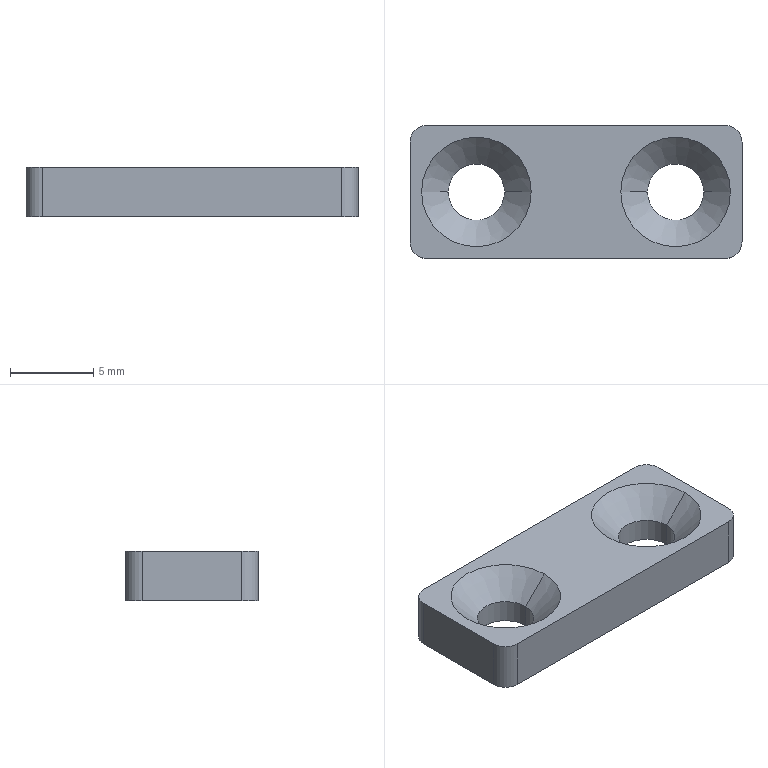Part | STEP file | 03-19 sensor press plate | 1 solid | 18 faces | box 20 x 8 x 3 mm | volume 387.026 mm3 | cylinder 8 | plane 6 | cone 4 | commonest cylinder face diameters 2 x4 3.4 x4
STEP:
#1=CARTESIAN_POINT('',(-7.7,0.,1.4));
#2=VERTEX_POINT('',#1);
#3=CARTESIAN_POINT('',(-4.3,0.,1.4));
#4=VERTEX_POINT('',#3);
#5=CARTESIAN_POINT('',(-6.,0.,1.4));
#6=DIRECTION('',(0.,0.,1.));
#7=DIRECTION('',(1.,0.,0.));
#8=AXIS2_PLACEMENT_3D('',#5,#6,#7);
#9=CIRCLE('',#8,1.7);
#10=EDGE_CURVE('',#2,#4,#9,.T.);
#11=ORIENTED_EDGE('',*,*,#10,.F.);
#12=CARTESIAN_POINT('',(-9.3,0.,3.));
#13=VERTEX_POINT('',#12);
#14=CARTESIAN_POINT('',(-9.3,0.,3.));
#15=DIRECTION('',(-0.7071,0.,0.7071));
#16=VECTOR('',#15,1000.);
#17=LINE('',#14,#16);
#18=EDGE_CURVE('',#2,#13,#17,.T.);
#19=ORIENTED_EDGE('',*,*,#18,.T.);
#20=CARTESIAN_POINT('',(-2.7,0.,3.));
#21=VERTEX_POINT('',#20);
#22=CARTESIAN_POINT('',(-6.,0.,3.));
#23=DIRECTION('',(0.,0.,1.));
#24=DIRECTION('',(1.,0.,0.));
#25=AXIS2_PLACEMENT_3D('',#22,#23,#24);
#26=CIRCLE('',#25,3.3);
#27=EDGE_CURVE('',#13,#21,#26,.T.);
#28=ORIENTED_EDGE('',*,*,#27,.T.);
#29=CARTESIAN_POINT('',(-2.7,0.,3.));
#30=DIRECTION('',(0.7071,0.,0.7071));
#31=VECTOR('',#30,1000.);
#32=LINE('',#29,#31);
#33=EDGE_CURVE('',#4,#21,#32,.T.);
#34=ORIENTED_EDGE('',*,*,#33,.F.);
#35=EDGE_LOOP('',(#11,#19,#28,#34));
#36=FACE_OUTER_BOUND('',#35,.T.);
#37=CARTESIAN_POINT('',(-6.,0.,3.));
#38=DIRECTION('',(0.,0.,1.));
#39=DIRECTION('',(1.,0.,0.));
#40=AXIS2_PLACEMENT_3D('',#37,#38,#39);
#41=CONICAL_SURFACE('',#40,3.3,0.7854);
#42=ADVANCED_FACE('',(#36),#41,.F.);
#43=CARTESIAN_POINT('',(-7.7,0.,0.));
#44=VERTEX_POINT('',#43);
#45=CARTESIAN_POINT('',(-4.3,0.,0.));
#46=VERTEX_POINT('',#45);
#47=CARTESIAN_POINT('',(-6.,0.,0.));
#48=DIRECTION('',(0.,0.,1.));
#49=DIRECTION('',(1.,0.,0.));
#50=AXIS2_PLACEMENT_3D('',#47,#48,#49);
#51=CIRCLE('',#50,1.7);
#52=EDGE_CURVE('',#44,#46,#51,.T.);
#53=ORIENTED_EDGE('',*,*,#52,.F.);
#54=CARTESIAN_POINT('',(-7.7,0.,3.));
#55=DIRECTION('',(0.,0.,1.));
#56=VECTOR('',#55,1000.);
#57=LINE('',#54,#56);
#58=EDGE_CURVE('',#44,#2,#57,.T.);
#59=ORIENTED_EDGE('',*,*,#58,.T.);
#60=ORIENTED_EDGE('',*,*,#10,.T.);
#61=CARTESIAN_POINT('',(-4.3,0.,3.));
#62=DIRECTION('',(0.,0.,1.));
#63=VECTOR('',#62,1000.);
#64=LINE('',#61,#63);
#65=EDGE_CURVE('',#46,#4,#64,.T.);
#66=ORIENTED_EDGE('',*,*,#65,.F.);
#67=EDGE_LOOP('',(#53,#59,#60,#66));
#68=FACE_OUTER_BOUND('',#67,.T.);
#69=CARTESIAN_POINT('',(-6.,0.,3.));
#70=DIRECTION('',(0.,0.,1.));
#71=DIRECTION('',(1.,0.,0.));
#72=AXIS2_PLACEMENT_3D('',#69,#70,#71);
#73=CYLINDRICAL_SURFACE('',#72,1.7);
#74=ADVANCED_FACE('',(#68),#73,.F.);
#75=CARTESIAN_POINT('',(4.3,0.,1.4));
#76=VERTEX_POINT('',#75);
#77=CARTESIAN_POINT('',(7.7,0.,1.4));
#78=VERTEX_POINT('',#77);
#79=CARTESIAN_POINT('',(6.,0.,1.4));
#80=DIRECTION('',(0.,0.,1.));
#81=DIRECTION('',(1.,0.,0.));
#82=AXIS2_PLACEMENT_3D('',#79,#80,#81);
#83=CIRCLE('',#82,1.7);
#84=EDGE_CURVE('',#76,#78,#83,.T.);
#85=ORIENTED_EDGE('',*,*,#84,.F.);
#86=CARTESIAN_POINT('',(2.7,0.,3.));
#87=VERTEX_POINT('',#86);
#88=CARTESIAN_POINT('',(2.7,0.,3.));
#89=DIRECTION('',(-0.7071,0.,0.7071));
#90=VECTOR('',#89,1000.);
#91=LINE('',#88,#90);
#92=EDGE_CURVE('',#76,#87,#91,.T.);
#93=ORIENTED_EDGE('',*,*,#92,.T.);
#94=CARTESIAN_POINT('',(9.3,0.,3.));
#95=VERTEX_POINT('',#94);
#96=CARTESIAN_POINT('',(6.,0.,3.));
#97=DIRECTION('',(0.,0.,1.));
#98=DIRECTION('',(1.,0.,0.));
#99=AXIS2_PLACEMENT_3D('',#96,#97,#98);
#100=CIRCLE('',#99,3.3);
#101=EDGE_CURVE('',#87,#95,#100,.T.);
#102=ORIENTED_EDGE('',*,*,#101,.T.);
#103=CARTESIAN_POINT('',(9.3,0.,3.));
#104=DIRECTION('',(0.7071,0.,0.7071));
#105=VECTOR('',#104,1000.);
#106=LINE('',#103,#105);
#107=EDGE_CURVE('',#78,#95,#106,.T.);
#108=ORIENTED_EDGE('',*,*,#107,.F.);
#109=EDGE_LOOP('',(#85,#93,#102,#108));
#110=FACE_OUTER_BOUND('',#109,.T.);
#111=CARTESIAN_POINT('',(6.,0.,3.));
#112=DIRECTION('',(0.,0.,1.));
#113=DIRECTION('',(1.,0.,0.));
#114=AXIS2_PLACEMENT_3D('',#111,#112,#113);
#115=CONICAL_SURFACE('',#114,3.3,0.7854);
#116=ADVANCED_FACE('',(#110),#115,.F.);
#117=CARTESIAN_POINT('',(4.3,0.,0.));
#118=VERTEX_POINT('',#117);
#119=CARTESIAN_POINT('',(7.7,0.,0.));
#120=VERTEX_POINT('',#119);
#121=CARTESIAN_POINT('',(6.,0.,0.));
#122=DIRECTION('',(0.,0.,1.));
#123=DIRECTION('',(1.,0.,0.));
#124=AXIS2_PLACEMENT_3D('',#121,#122,#123);
#125=CIRCLE('',#124,1.7);
#126=EDGE_CURVE('',#118,#120,#125,.T.);
#127=ORIENTED_EDGE('',*,*,#126,.F.);
#128=CARTESIAN_POINT('',(4.3,0.,3.));
#129=DIRECTION('',(0.,0.,1.));
#130=VECTOR('',#129,1000.);
#131=LINE('',#128,#130);
#132=EDGE_CURVE('',#118,#76,#131,.T.);
#133=ORIENTED_EDGE('',*,*,#132,.T.);
#134=ORIENTED_EDGE('',*,*,#84,.T.);
#135=CARTESIAN_POINT('',(7.7,0.,3.));
#136=DIRECTION('',(0.,0.,1.));
#137=VECTOR('',#136,1000.);
#138=LINE('',#135,#137);
#139=EDGE_CURVE('',#120,#78,#138,.T.);
#140=ORIENTED_EDGE('',*,*,#139,.F.);
#141=EDGE_LOOP('',(#127,#133,#134,#140));
#142=FACE_OUTER_BOUND('',#141,.T.);
#143=CARTESIAN_POINT('',(6.,0.,3.));
#144=DIRECTION('',(0.,0.,1.));
#145=DIRECTION('',(1.,0.,0.));
#146=AXIS2_PLACEMENT_3D('',#143,#144,#145);
#147=CYLINDRICAL_SURFACE('',#146,1.7);
#148=ADVANCED_FACE('',(#142),#147,.F.);
#149=CARTESIAN_POINT('',(10.,-3.,3.));
#150=VERTEX_POINT('',#149);
#151=CARTESIAN_POINT('',(10.,3.,3.));
#152=VERTEX_POINT('',#151);
#153=CARTESIAN_POINT('',(10.,4.,3.));
#154=DIRECTION('',(0.,1.,0.));
#155=VECTOR('',#154,1000.);
#156=LINE('',#153,#155);
#157=EDGE_CURVE('',#150,#152,#156,.T.);
#158=ORIENTED_EDGE('',*,*,#157,.F.);
#159=CARTESIAN_POINT('',(10.,-3.,0.));
#160=VERTEX_POINT('',#159);
#161=CARTESIAN_POINT('',(10.,-3.,3.));
#162=DIRECTION('',(0.,0.,-1.));
#163=VECTOR('',#162,1000.);
#164=LINE('',#161,#163);
#165=EDGE_CURVE('',#150,#160,#164,.T.);
#166=ORIENTED_EDGE('',*,*,#165,.T.);
#167=CARTESIAN_POINT('',(10.,3.,0.));
#168=VERTEX_POINT('',#167);
#169=CARTESIAN_POINT('',(10.,4.,0.));
#170=DIRECTION('',(0.,1.,0.));
#171=VECTOR('',#170,1000.);
#172=LINE('',#169,#171);
#173=EDGE_CURVE('',#160,#168,#172,.T.);
#174=ORIENTED_EDGE('',*,*,#173,.T.);
#175=CARTESIAN_POINT('',(10.,3.,3.));
#176=DIRECTION('',(0.,0.,1.));
#177=VECTOR('',#176,1000.);
#178=LINE('',#175,#177);
#179=EDGE_CURVE('',#168,#152,#178,.T.);
#180=ORIENTED_EDGE('',*,*,#179,.T.);
#181=EDGE_LOOP('',(#158,#166,#174,#180));
#182=FACE_OUTER_BOUND('',#181,.T.);
#183=CARTESIAN_POINT('',(10.,4.,3.));
#184=DIRECTION('',(-1.,0.,0.));
#185=DIRECTION('',(0.,-1.,0.));
#186=AXIS2_PLACEMENT_3D('',#183,#184,#185);
#187=PLANE('',#186);
#188=ADVANCED_FACE('',(#182),#187,.F.);
#189=CARTESIAN_POINT('',(9.,4.,3.));
#190=VERTEX_POINT('',#189);
#191=CARTESIAN_POINT('',(-9.,4.,3.));
#192=VERTEX_POINT('',#191);
#193=CARTESIAN_POINT('',(-10.,4.,3.));
#194=DIRECTION('',(-1.,0.,0.));
#195=VECTOR('',#194,1000.);
#196=LINE('',#193,#195);
#197=EDGE_CURVE('',#190,#192,#196,.T.);
#198=ORIENTED_EDGE('',*,*,#197,.F.);
#199=CARTESIAN_POINT('',(9.,4.,0.));
#200=VERTEX_POINT('',#199);
#201=CARTESIAN_POINT('',(9.,4.,3.));
#202=DIRECTION('',(0.,0.,-1.));
#203=VECTOR('',#202,1000.);
#204=LINE('',#201,#203);
#205=EDGE_CURVE('',#190,#200,#204,.T.);
#206=ORIENTED_EDGE('',*,*,#205,.T.);
#207=CARTESIAN_POINT('',(-9.,4.,0.));
#208=VERTEX_POINT('',#207);
#209=CARTESIAN_POINT('',(-10.,4.,0.));
#210=DIRECTION('',(-1.,0.,0.));
#211=VECTOR('',#210,1000.);
#212=LINE('',#209,#211);
#213=EDGE_CURVE('',#200,#208,#212,.T.);
#214=ORIENTED_EDGE('',*,*,#213,.T.);
#215=CARTESIAN_POINT('',(-9.,4.,3.));
#216=DIRECTION('',(0.,0.,1.));
#217=VECTOR('',#216,1000.);
#218=LINE('',#215,#217);
#219=EDGE_CURVE('',#208,#192,#218,.T.);
#220=ORIENTED_EDGE('',*,*,#219,.T.);
#221=EDGE_LOOP('',(#198,#206,#214,#220));
#222=FACE_OUTER_BOUND('',#221,.T.);
#223=CARTESIAN_POINT('',(-10.,4.,3.));
#224=DIRECTION('',(0.,-1.,0.));
#225=DIRECTION('',(0.,0.,-1.));
#226=AXIS2_PLACEMENT_3D('',#223,#224,#225);
#227=PLANE('',#226);
#228=ADVANCED_FACE('',(#222),#227,.F.);
#229=CARTESIAN_POINT('',(-10.,3.,0.));
#230=VERTEX_POINT('',#229);
#231=CARTESIAN_POINT('',(-10.,-3.,0.));
#232=VERTEX_POINT('',#231);
#233=CARTESIAN_POINT('',(-10.,4.,0.));
#234=DIRECTION('',(0.,-1.,0.));
#235=VECTOR('',#234,1000.);
#236=LINE('',#233,#235);
#237=EDGE_CURVE('',#230,#232,#236,.T.);
#238=ORIENTED_EDGE('',*,*,#237,.T.);
#239=CARTESIAN_POINT('',(-10.,-3.,3.));
#240=VERTEX_POINT('',#239);
#241=CARTESIAN_POINT('',(-10.,-3.,3.));
#242=DIRECTION('',(0.,0.,1.));
#243=VECTOR('',#242,1000.);
#244=LINE('',#241,#243);
#245=EDGE_CURVE('',#232,#240,#244,.T.);
#246=ORIENTED_EDGE('',*,*,#245,.T.);
#247=CARTESIAN_POINT('',(-10.,3.,3.));
#248=VERTEX_POINT('',#247);
#249=CARTESIAN_POINT('',(-10.,4.,3.));
#250=DIRECTION('',(0.,-1.,0.));
#251=VECTOR('',#250,1000.);
#252=LINE('',#249,#251);
#253=EDGE_CURVE('',#248,#240,#252,.T.);
#254=ORIENTED_EDGE('',*,*,#253,.F.);
#255=CARTESIAN_POINT('',(-10.,3.,3.));
#256=DIRECTION('',(0.,0.,-1.));
#257=VECTOR('',#256,1000.);
#258=LINE('',#255,#257);
#259=EDGE_CURVE('',#248,#230,#258,.T.);
#260=ORIENTED_EDGE('',*,*,#259,.T.);
#261=EDGE_LOOP('',(#238,#246,#254,#260));
#262=FACE_OUTER_BOUND('',#261,.T.);
#263=CARTESIAN_POINT('',(-10.,4.,3.));
#264=DIRECTION('',(1.,0.,0.));
#265=DIRECTION('',(0.,1.,0.));
#266=AXIS2_PLACEMENT_3D('',#263,#264,#265);
#267=PLANE('',#266);
#268=ADVANCED_FACE('',(#262),#267,.F.);
#269=CARTESIAN_POINT('',(-9.,-4.,0.));
#270=VERTEX_POINT('',#269);
#271=CARTESIAN_POINT('',(9.,-4.,0.));
#272=VERTEX_POINT('',#271);
#273=CARTESIAN_POINT('',(-10.,-4.,0.));
#274=DIRECTION('',(1.,0.,0.));
#275=VECTOR('',#274,1000.);
#276=LINE('',#273,#275);
#277=EDGE_CURVE('',#270,#272,#276,.T.);
#278=ORIENTED_EDGE('',*,*,#277,.T.);
#279=CARTESIAN_POINT('',(9.,-4.,3.));
#280=VERTEX_POINT('',#279);
#281=CARTESIAN_POINT('',(9.,-4.,3.));
#282=DIRECTION('',(0.,0.,1.));
#283=VECTOR('',#282,1000.);
#284=LINE('',#281,#283);
#285=EDGE_CURVE('',#272,#280,#284,.T.);
#286=ORIENTED_EDGE('',*,*,#285,.T.);
#287=CARTESIAN_POINT('',(-9.,-4.,3.));
#288=VERTEX_POINT('',#287);
#289=CARTESIAN_POINT('',(-10.,-4.,3.));
#290=DIRECTION('',(1.,0.,0.));
#291=VECTOR('',#290,1000.);
#292=LINE('',#289,#291);
#293=EDGE_CURVE('',#288,#280,#292,.T.);
#294=ORIENTED_EDGE('',*,*,#293,.F.);
#295=CARTESIAN_POINT('',(-9.,-4.,3.));
#296=DIRECTION('',(0.,0.,-1.));
#297=VECTOR('',#296,1000.);
#298=LINE('',#295,#297);
#299=EDGE_CURVE('',#288,#270,#298,.T.);
#300=ORIENTED_EDGE('',*,*,#299,.T.);
#301=EDGE_LOOP('',(#278,#286,#294,#300));
#302=FACE_OUTER_BOUND('',#301,.T.);
#303=CARTESIAN_POINT('',(-10.,-4.,3.));
#304=DIRECTION('',(0.,1.,0.));
#305=DIRECTION('',(0.,0.,1.));
#306=AXIS2_PLACEMENT_3D('',#303,#304,#305);
#307=PLANE('',#306);
#308=ADVANCED_FACE('',(#302),#307,.F.);
#309=CARTESIAN_POINT('',(-6.,0.,3.));
#310=DIRECTION('',(0.,0.,1.));
#311=DIRECTION('',(1.,0.,0.));
#312=AXIS2_PLACEMENT_3D('',#309,#310,#311);
#313=CIRCLE('',#312,3.3);
#314=EDGE_CURVE('',#21,#13,#313,.T.);
#315=ORIENTED_EDGE('',*,*,#314,.F.);
#316=ORIENTED_EDGE('',*,*,#27,.F.);
#317=EDGE_LOOP('',(#315,#316));
#318=FACE_BOUND('',#317,.T.);
#319=CARTESIAN_POINT('',(6.,0.,3.));
#320=DIRECTION('',(0.,0.,1.));
#321=DIRECTION('',(1.,0.,0.));
#322=AXIS2_PLACEMENT_3D('',#319,#320,#321);
#323=CIRCLE('',#322,3.3);
#324=EDGE_CURVE('',#95,#87,#323,.T.);
#325=ORIENTED_EDGE('',*,*,#324,.F.);
#326=ORIENTED_EDGE('',*,*,#101,.F.);
#327=EDGE_LOOP('',(#325,#326));
#328=FACE_BOUND('',#327,.T.);
#329=ORIENTED_EDGE('',*,*,#293,.T.);
#330=CARTESIAN_POINT('',(9.,-3.,3.));
#331=DIRECTION('',(0.,0.,1.));
#332=DIRECTION('',(1.,0.,0.));
#333=AXIS2_PLACEMENT_3D('',#330,#331,#332);
#334=CIRCLE('',#333,1.);
#335=EDGE_CURVE('',#280,#150,#334,.T.);
#336=ORIENTED_EDGE('',*,*,#335,.T.);
#337=ORIENTED_EDGE('',*,*,#157,.T.);
#338=CARTESIAN_POINT('',(9.,3.,3.));
#339=DIRECTION('',(0.,0.,1.));
#340=DIRECTION('',(1.,0.,0.));
#341=AXIS2_PLACEMENT_3D('',#338,#339,#340);
#342=CIRCLE('',#341,1.);
#343=EDGE_CURVE('',#152,#190,#342,.T.);
#344=ORIENTED_EDGE('',*,*,#343,.T.);
#345=ORIENTED_EDGE('',*,*,#197,.T.);
#346=CARTESIAN_POINT('',(-9.,3.,3.));
#347=DIRECTION('',(0.,0.,1.));
#348=DIRECTION('',(1.,0.,0.));
#349=AXIS2_PLACEMENT_3D('',#346,#347,#348);
#350=CIRCLE('',#349,1.);
#351=EDGE_CURVE('',#192,#248,#350,.T.);
#352=ORIENTED_EDGE('',*,*,#351,.T.);
#353=ORIENTED_EDGE('',*,*,#253,.T.);
#354=CARTESIAN_POINT('',(-9.,-3.,3.));
#355=DIRECTION('',(0.,0.,1.));
#356=DIRECTION('',(1.,0.,0.));
#357=AXIS2_PLACEMENT_3D('',#354,#355,#356);
#358=CIRCLE('',#357,1.);
#359=EDGE_CURVE('',#240,#288,#358,.T.);
#360=ORIENTED_EDGE('',*,*,#359,.T.);
#361=EDGE_LOOP('',(#329,#336,#337,#344,#345,#352,#353,#360));
#362=FACE_OUTER_BOUND('',#361,.T.);
#363=CARTESIAN_POINT('',(10.,-4.,3.));
#364=DIRECTION('',(0.,0.,1.));
#365=DIRECTION('',(1.,0.,0.));
#366=AXIS2_PLACEMENT_3D('',#363,#364,#365);
#367=PLANE('',#366);
#368=ADVANCED_FACE('',(#318,#328,#362),#367,.T.);
#369=CARTESIAN_POINT('',(-6.,0.,0.));
#370=DIRECTION('',(0.,0.,1.));
#371=DIRECTION('',(1.,0.,0.));
#372=AXIS2_PLACEMENT_3D('',#369,#370,#371);
#373=CIRCLE('',#372,1.7);
#374=EDGE_CURVE('',#46,#44,#373,.T.);
#375=ORIENTED_EDGE('',*,*,#374,.T.);
#376=ORIENTED_EDGE('',*,*,#52,.T.);
#377=EDGE_LOOP('',(#375,#376));
#378=FACE_BOUND('',#377,.T.);
#379=CARTESIAN_POINT('',(6.,0.,0.));
#380=DIRECTION('',(0.,0.,1.));
#381=DIRECTION('',(1.,0.,0.));
#382=AXIS2_PLACEMENT_3D('',#379,#380,#381);
#383=CIRCLE('',#382,1.7);
#384=EDGE_CURVE('',#120,#118,#383,.T.);
#385=ORIENTED_EDGE('',*,*,#384,.T.);
#386=ORIENTED_EDGE('',*,*,#126,.T.);
#387=EDGE_LOOP('',(#385,#386));
#388=FACE_BOUND('',#387,.T.);
#389=ORIENTED_EDGE('',*,*,#173,.F.);
#390=CARTESIAN_POINT('',(9.,-3.,0.));
#391=DIRECTION('',(0.,0.,-1.));
#392=DIRECTION('',(1.,0.,0.));
#393=AXIS2_PLACEMENT_3D('',#390,#391,#392);
#394=CIRCLE('',#393,1.);
#395=EDGE_CURVE('',#160,#272,#394,.T.);
#396=ORIENTED_EDGE('',*,*,#395,.T.);
#397=ORIENTED_EDGE('',*,*,#277,.F.);
#398=CARTESIAN_POINT('',(-9.,-3.,0.));
#399=DIRECTION('',(0.,0.,-1.));
#400=DIRECTION('',(1.,0.,0.));
#401=AXIS2_PLACEMENT_3D('',#398,#399,#400);
#402=CIRCLE('',#401,1.);
#403=EDGE_CURVE('',#270,#232,#402,.T.);
#404=ORIENTED_EDGE('',*,*,#403,.T.);
#405=ORIENTED_EDGE('',*,*,#237,.F.);
#406=CARTESIAN_POINT('',(-9.,3.,0.));
#407=DIRECTION('',(0.,0.,-1.));
#408=DIRECTION('',(1.,0.,0.));
#409=AXIS2_PLACEMENT_3D('',#406,#407,#408);
#410=CIRCLE('',#409,1.);
#411=EDGE_CURVE('',#230,#208,#410,.T.);
#412=ORIENTED_EDGE('',*,*,#411,.T.);
#413=ORIENTED_EDGE('',*,*,#213,.F.);
#414=CARTESIAN_POINT('',(9.,3.,0.));
#415=DIRECTION('',(0.,0.,-1.));
#416=DIRECTION('',(1.,0.,0.));
#417=AXIS2_PLACEMENT_3D('',#414,#415,#416);
#418=CIRCLE('',#417,1.);
#419=EDGE_CURVE('',#200,#168,#418,.T.);
#420=ORIENTED_EDGE('',*,*,#419,.T.);
#421=EDGE_LOOP('',(#389,#396,#397,#404,#405,#412,#413,#420));
#422=FACE_OUTER_BOUND('',#421,.T.);
#423=CARTESIAN_POINT('',(10.,-4.,0.));
#424=DIRECTION('',(0.,0.,1.));
#425=DIRECTION('',(1.,0.,0.));
#426=AXIS2_PLACEMENT_3D('',#423,#424,#425);
#427=PLANE('',#426);
#428=ADVANCED_FACE('',(#378,#388,#422),#427,.F.);
#429=ORIENTED_EDGE('',*,*,#335,.F.);
#430=ORIENTED_EDGE('',*,*,#285,.F.);
#431=ORIENTED_EDGE('',*,*,#395,.F.);
#432=ORIENTED_EDGE('',*,*,#165,.F.);
#433=EDGE_LOOP('',(#429,#430,#431,#432));
#434=FACE_OUTER_BOUND('',#433,.T.);
#435=CARTESIAN_POINT('',(9.,-3.,3.));
#436=DIRECTION('',(0.,0.,-1.));
#437=DIRECTION('',(-1.,0.,0.));
#438=AXIS2_PLACEMENT_3D('',#435,#436,#437);
#439=CYLINDRICAL_SURFACE('',#438,1.);
#440=ADVANCED_FACE('',(#434),#439,.T.);
#441=ORIENTED_EDGE('',*,*,#359,.F.);
#442=ORIENTED_EDGE('',*,*,#245,.F.);
#443=ORIENTED_EDGE('',*,*,#403,.F.);
#444=ORIENTED_EDGE('',*,*,#299,.F.);
#445=EDGE_LOOP('',(#441,#442,#443,#444));
#446=FACE_OUTER_BOUND('',#445,.T.);
#447=CARTESIAN_POINT('',(-9.,-3.,3.));
#448=DIRECTION('',(0.,0.,-1.));
#449=DIRECTION('',(-1.,0.,0.));
#450=AXIS2_PLACEMENT_3D('',#447,#448,#449);
#451=CYLINDRICAL_SURFACE('',#450,1.);
#452=ADVANCED_FACE('',(#446),#451,.T.);
#453=ORIENTED_EDGE('',*,*,#343,.F.);
#454=ORIENTED_EDGE('',*,*,#179,.F.);
#455=ORIENTED_EDGE('',*,*,#419,.F.);
#456=ORIENTED_EDGE('',*,*,#205,.F.);
#457=EDGE_LOOP('',(#453,#454,#455,#456));
#458=FACE_OUTER_BOUND('',#457,.T.);
#459=CARTESIAN_POINT('',(9.,3.,3.));
#460=DIRECTION('',(0.,0.,-1.));
#461=DIRECTION('',(-1.,0.,0.));
#462=AXIS2_PLACEMENT_3D('',#459,#460,#461);
#463=CYLINDRICAL_SURFACE('',#462,1.);
#464=ADVANCED_FACE('',(#458),#463,.T.);
#465=ORIENTED_EDGE('',*,*,#351,.F.);
#466=ORIENTED_EDGE('',*,*,#219,.F.);
#467=ORIENTED_EDGE('',*,*,#411,.F.);
#468=ORIENTED_EDGE('',*,*,#259,.F.);
#469=EDGE_LOOP('',(#465,#466,#467,#468));
#470=FACE_OUTER_BOUND('',#469,.T.);
#471=CARTESIAN_POINT('',(-9.,3.,3.));
#472=DIRECTION('',(0.,0.,-1.));
#473=DIRECTION('',(-1.,0.,0.));
#474=AXIS2_PLACEMENT_3D('',#471,#472,#473);
#475=CYLINDRICAL_SURFACE('',#474,1.);
#476=ADVANCED_FACE('',(#470),#475,.T.);
#477=ORIENTED_EDGE('',*,*,#132,.F.);
#478=ORIENTED_EDGE('',*,*,#384,.F.);
#479=ORIENTED_EDGE('',*,*,#139,.T.);
#480=CARTESIAN_POINT('',(6.,0.,1.4));
#481=DIRECTION('',(0.,0.,1.));
#482=DIRECTION('',(1.,0.,0.));
#483=AXIS2_PLACEMENT_3D('',#480,#481,#482);
#484=CIRCLE('',#483,1.7);
#485=EDGE_CURVE('',#78,#76,#484,.T.);
#486=ORIENTED_EDGE('',*,*,#485,.T.);
#487=EDGE_LOOP('',(#477,#478,#479,#486));
#488=FACE_OUTER_BOUND('',#487,.T.);
#489=CARTESIAN_POINT('',(6.,0.,3.));
#490=DIRECTION('',(0.,0.,1.));
#491=DIRECTION('',(1.,0.,0.));
#492=AXIS2_PLACEMENT_3D('',#489,#490,#491);
#493=CYLINDRICAL_SURFACE('',#492,1.7);
#494=ADVANCED_FACE('',(#488),#493,.F.);
#495=ORIENTED_EDGE('',*,*,#92,.F.);
#496=ORIENTED_EDGE('',*,*,#485,.F.);
#497=ORIENTED_EDGE('',*,*,#107,.T.);
#498=ORIENTED_EDGE('',*,*,#324,.T.);
#499=EDGE_LOOP('',(#495,#496,#497,#498));
#500=FACE_OUTER_BOUND('',#499,.T.);
#501=CARTESIAN_POINT('',(6.,0.,3.));
#502=DIRECTION('',(0.,0.,1.));
#503=DIRECTION('',(1.,0.,0.));
#504=AXIS2_PLACEMENT_3D('',#501,#502,#503);
#505=CONICAL_SURFACE('',#504,3.3,0.7854);
#506=ADVANCED_FACE('',(#500),#505,.F.);
#507=ORIENTED_EDGE('',*,*,#58,.F.);
#508=ORIENTED_EDGE('',*,*,#374,.F.);
#509=ORIENTED_EDGE('',*,*,#65,.T.);
#510=CARTESIAN_POINT('',(-6.,0.,1.4));
#511=DIRECTION('',(0.,0.,1.));
#512=DIRECTION('',(1.,0.,0.));
#513=AXIS2_PLACEMENT_3D('',#510,#511,#512);
#514=CIRCLE('',#513,1.7);
#515=EDGE_CURVE('',#4,#2,#514,.T.);
#516=ORIENTED_EDGE('',*,*,#515,.T.);
#517=EDGE_LOOP('',(#507,#508,#509,#516));
#518=FACE_OUTER_BOUND('',#517,.T.);
#519=CARTESIAN_POINT('',(-6.,0.,3.));
#520=DIRECTION('',(0.,0.,1.));
#521=DIRECTION('',(1.,0.,0.));
#522=AXIS2_PLACEMENT_3D('',#519,#520,#521);
#523=CYLINDRICAL_SURFACE('',#522,1.7);
#524=ADVANCED_FACE('',(#518),#523,.F.);
#525=ORIENTED_EDGE('',*,*,#18,.F.);
#526=ORIENTED_EDGE('',*,*,#515,.F.);
#527=ORIENTED_EDGE('',*,*,#33,.T.);
#528=ORIENTED_EDGE('',*,*,#314,.T.);
#529=EDGE_LOOP('',(#525,#526,#527,#528));
#530=FACE_OUTER_BOUND('',#529,.T.);
#531=CARTESIAN_POINT('',(-6.,0.,3.));
#532=DIRECTION('',(0.,0.,1.));
#533=DIRECTION('',(1.,0.,0.));
#534=AXIS2_PLACEMENT_3D('',#531,#532,#533);
#535=CONICAL_SURFACE('',#534,3.3,0.7854);
#536=ADVANCED_FACE('',(#530),#535,.F.);
#537=CLOSED_SHELL('',(#42,#74,#116,#148,#188,#228,#268,#308,#368,#428,#440,#452,#464,#476,#494,#506,#524,#536));
#538=MANIFOLD_SOLID_BREP('',#537);
#539=CARTESIAN_POINT('',(0.,0.,0.));
#540=DIRECTION('',(0.,0.,1.));
#541=DIRECTION('',(1.,0.,0.));
#542=AXIS2_PLACEMENT_3D('',#539,#540,#541);
#543=(LENGTH_UNIT()NAMED_UNIT(*)SI_UNIT(.MILLI.,.METRE.));
#544=UNCERTAINTY_MEASURE_WITH_UNIT(LENGTH_MEASURE(0.00001),#543,'','');
#545=(NAMED_UNIT(*)PLANE_ANGLE_UNIT()SI_UNIT($,.RADIAN.));
#546=(NAMED_UNIT(*)SI_UNIT($,.STERADIAN.)SOLID_ANGLE_UNIT());
#547=(GEOMETRIC_REPRESENTATION_CONTEXT(3)GLOBAL_UNCERTAINTY_ASSIGNED_CONTEXT((#544))GLOBAL_UNIT_ASSIGNED_CONTEXT((#543,#545,#546))REPRESENTATION_CONTEXT('',''));
#548=ADVANCED_BREP_SHAPE_REPRESENTATION('',(#538,#542),#547);